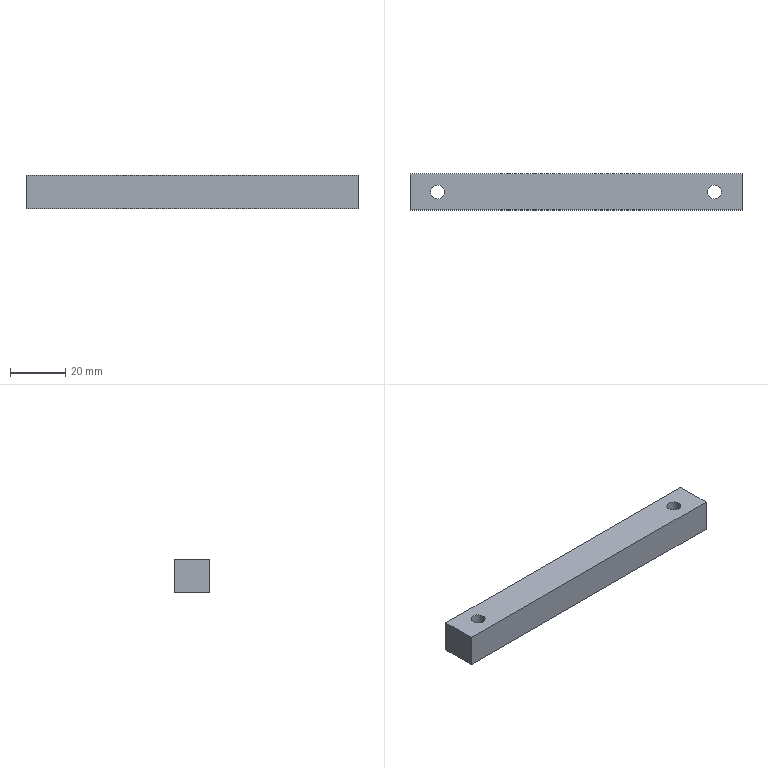Part | STEP file | [14] | 1 solid | 10 faces | box 120 x 13 x 12 mm | volume 18249 mm3 | plane 6 | cylinder 4 | commonest cylinder face diameters 5 x4
STEP:
#1=CARTESIAN_POINT('',(107.5,6.5,12.));
#2=VERTEX_POINT('',#1);
#3=CARTESIAN_POINT('',(112.5,6.5,12.));
#4=VERTEX_POINT('',#3);
#5=CARTESIAN_POINT('',(110.,6.5,12.));
#6=DIRECTION('',(0.,0.,-1.));
#7=DIRECTION('',(1.,0.,0.));
#8=AXIS2_PLACEMENT_3D('',#5,#6,#7);
#9=CIRCLE('',#8,2.5);
#10=EDGE_CURVE('',#2,#4,#9,.T.);
#11=ORIENTED_EDGE('',*,*,#10,.F.);
#12=CARTESIAN_POINT('',(107.5,6.5,0.));
#13=VERTEX_POINT('',#12);
#14=CARTESIAN_POINT('',(107.5,6.5,12.));
#15=DIRECTION('',(0.,0.,-1.));
#16=VECTOR('',#15,1000.);
#17=LINE('',#14,#16);
#18=EDGE_CURVE('',#2,#13,#17,.T.);
#19=ORIENTED_EDGE('',*,*,#18,.T.);
#20=CARTESIAN_POINT('',(112.5,6.5,0.));
#21=VERTEX_POINT('',#20);
#22=CARTESIAN_POINT('',(110.,6.5,0.));
#23=DIRECTION('',(0.,0.,1.));
#24=DIRECTION('',(-1.,0.,0.));
#25=AXIS2_PLACEMENT_3D('',#22,#23,#24);
#26=CIRCLE('',#25,2.5);
#27=EDGE_CURVE('',#21,#13,#26,.T.);
#28=ORIENTED_EDGE('',*,*,#27,.F.);
#29=CARTESIAN_POINT('',(112.5,6.5,12.));
#30=DIRECTION('',(0.,0.,-1.));
#31=VECTOR('',#30,1000.);
#32=LINE('',#29,#31);
#33=EDGE_CURVE('',#4,#21,#32,.T.);
#34=ORIENTED_EDGE('',*,*,#33,.F.);
#35=EDGE_LOOP('',(#11,#19,#28,#34));
#36=FACE_OUTER_BOUND('',#35,.T.);
#37=CARTESIAN_POINT('',(110.,6.5,12.));
#38=DIRECTION('',(0.,0.,-1.));
#39=DIRECTION('',(1.,0.,0.));
#40=AXIS2_PLACEMENT_3D('',#37,#38,#39);
#41=CYLINDRICAL_SURFACE('',#40,2.5);
#42=ADVANCED_FACE('',(#36),#41,.F.);
#43=CARTESIAN_POINT('',(7.5,6.5,12.));
#44=VERTEX_POINT('',#43);
#45=CARTESIAN_POINT('',(12.5,6.5,12.));
#46=VERTEX_POINT('',#45);
#47=CARTESIAN_POINT('',(10.,6.5,12.));
#48=DIRECTION('',(0.,0.,-1.));
#49=DIRECTION('',(1.,0.,0.));
#50=AXIS2_PLACEMENT_3D('',#47,#48,#49);
#51=CIRCLE('',#50,2.5);
#52=EDGE_CURVE('',#44,#46,#51,.T.);
#53=ORIENTED_EDGE('',*,*,#52,.F.);
#54=CARTESIAN_POINT('',(7.5,6.5,0.));
#55=VERTEX_POINT('',#54);
#56=CARTESIAN_POINT('',(7.5,6.5,12.));
#57=DIRECTION('',(0.,0.,-1.));
#58=VECTOR('',#57,1000.);
#59=LINE('',#56,#58);
#60=EDGE_CURVE('',#44,#55,#59,.T.);
#61=ORIENTED_EDGE('',*,*,#60,.T.);
#62=CARTESIAN_POINT('',(12.5,6.5,0.));
#63=VERTEX_POINT('',#62);
#64=CARTESIAN_POINT('',(10.,6.5,0.));
#65=DIRECTION('',(0.,0.,1.));
#66=DIRECTION('',(-1.,0.,0.));
#67=AXIS2_PLACEMENT_3D('',#64,#65,#66);
#68=CIRCLE('',#67,2.5);
#69=EDGE_CURVE('',#63,#55,#68,.T.);
#70=ORIENTED_EDGE('',*,*,#69,.F.);
#71=CARTESIAN_POINT('',(12.5,6.5,12.));
#72=DIRECTION('',(0.,0.,-1.));
#73=VECTOR('',#72,1000.);
#74=LINE('',#71,#73);
#75=EDGE_CURVE('',#46,#63,#74,.T.);
#76=ORIENTED_EDGE('',*,*,#75,.F.);
#77=EDGE_LOOP('',(#53,#61,#70,#76));
#78=FACE_OUTER_BOUND('',#77,.T.);
#79=CARTESIAN_POINT('',(10.,6.5,12.));
#80=DIRECTION('',(0.,0.,-1.));
#81=DIRECTION('',(1.,0.,0.));
#82=AXIS2_PLACEMENT_3D('',#79,#80,#81);
#83=CYLINDRICAL_SURFACE('',#82,2.5);
#84=ADVANCED_FACE('',(#78),#83,.F.);
#85=CARTESIAN_POINT('',(0.,13.,0.));
#86=VERTEX_POINT('',#85);
#87=CARTESIAN_POINT('',(0.,13.,12.));
#88=VERTEX_POINT('',#87);
#89=CARTESIAN_POINT('',(0.,13.,6.));
#90=DIRECTION('',(0.,0.,1.));
#91=VECTOR('',#90,1000.);
#92=LINE('',#89,#91);
#93=EDGE_CURVE('',#86,#88,#92,.T.);
#94=ORIENTED_EDGE('',*,*,#93,.F.);
#95=CARTESIAN_POINT('',(0.,0.,0.));
#96=VERTEX_POINT('',#95);
#97=CARTESIAN_POINT('',(0.,6.5,0.));
#98=DIRECTION('',(0.,1.,0.));
#99=VECTOR('',#98,1000.);
#100=LINE('',#97,#99);
#101=EDGE_CURVE('',#96,#86,#100,.T.);
#102=ORIENTED_EDGE('',*,*,#101,.F.);
#103=CARTESIAN_POINT('',(0.,0.,12.));
#104=VERTEX_POINT('',#103);
#105=CARTESIAN_POINT('',(0.,0.,6.));
#106=DIRECTION('',(0.,0.,-1.));
#107=VECTOR('',#106,1000.);
#108=LINE('',#105,#107);
#109=EDGE_CURVE('',#104,#96,#108,.T.);
#110=ORIENTED_EDGE('',*,*,#109,.F.);
#111=CARTESIAN_POINT('',(0.,6.5,12.));
#112=DIRECTION('',(0.,-1.,0.));
#113=VECTOR('',#112,1000.);
#114=LINE('',#111,#113);
#115=EDGE_CURVE('',#88,#104,#114,.T.);
#116=ORIENTED_EDGE('',*,*,#115,.F.);
#117=EDGE_LOOP('',(#94,#102,#110,#116));
#118=FACE_OUTER_BOUND('',#117,.T.);
#119=CARTESIAN_POINT('',(0.,6.5,6.));
#120=DIRECTION('',(-1.,0.,0.));
#121=DIRECTION('',(0.,0.,-1.));
#122=AXIS2_PLACEMENT_3D('',#119,#120,#121);
#123=PLANE('',#122);
#124=ADVANCED_FACE('',(#118),#123,.T.);
#125=CARTESIAN_POINT('',(120.,13.,0.));
#126=VERTEX_POINT('',#125);
#127=CARTESIAN_POINT('',(120.,13.,0.));
#128=DIRECTION('',(-1.,0.,0.));
#129=VECTOR('',#128,1000.);
#130=LINE('',#127,#129);
#131=EDGE_CURVE('',#126,#86,#130,.T.);
#132=ORIENTED_EDGE('',*,*,#131,.T.);
#133=ORIENTED_EDGE('',*,*,#93,.T.);
#134=CARTESIAN_POINT('',(120.,13.,12.));
#135=VERTEX_POINT('',#134);
#136=CARTESIAN_POINT('',(120.,13.,12.));
#137=DIRECTION('',(-1.,0.,0.));
#138=VECTOR('',#137,1000.);
#139=LINE('',#136,#138);
#140=EDGE_CURVE('',#135,#88,#139,.T.);
#141=ORIENTED_EDGE('',*,*,#140,.F.);
#142=CARTESIAN_POINT('',(120.,13.,6.));
#143=DIRECTION('',(0.,0.,-1.));
#144=VECTOR('',#143,1000.);
#145=LINE('',#142,#144);
#146=EDGE_CURVE('',#135,#126,#145,.T.);
#147=ORIENTED_EDGE('',*,*,#146,.T.);
#148=EDGE_LOOP('',(#132,#133,#141,#147));
#149=FACE_OUTER_BOUND('',#148,.T.);
#150=CARTESIAN_POINT('',(120.,13.,6.));
#151=DIRECTION('',(0.,1.,0.));
#152=DIRECTION('',(1.,0.,0.));
#153=AXIS2_PLACEMENT_3D('',#150,#151,#152);
#154=PLANE('',#153);
#155=ADVANCED_FACE('',(#149),#154,.T.);
#156=CARTESIAN_POINT('',(110.,6.5,12.));
#157=DIRECTION('',(0.,0.,-1.));
#158=DIRECTION('',(1.,0.,0.));
#159=AXIS2_PLACEMENT_3D('',#156,#157,#158);
#160=CIRCLE('',#159,2.5);
#161=EDGE_CURVE('',#4,#2,#160,.T.);
#162=ORIENTED_EDGE('',*,*,#161,.T.);
#163=ORIENTED_EDGE('',*,*,#10,.T.);
#164=EDGE_LOOP('',(#162,#163));
#165=FACE_BOUND('',#164,.T.);
#166=CARTESIAN_POINT('',(10.,6.5,12.));
#167=DIRECTION('',(0.,0.,-1.));
#168=DIRECTION('',(1.,0.,0.));
#169=AXIS2_PLACEMENT_3D('',#166,#167,#168);
#170=CIRCLE('',#169,2.5);
#171=EDGE_CURVE('',#46,#44,#170,.T.);
#172=ORIENTED_EDGE('',*,*,#171,.T.);
#173=ORIENTED_EDGE('',*,*,#52,.T.);
#174=EDGE_LOOP('',(#172,#173));
#175=FACE_BOUND('',#174,.T.);
#176=ORIENTED_EDGE('',*,*,#140,.T.);
#177=ORIENTED_EDGE('',*,*,#115,.T.);
#178=CARTESIAN_POINT('',(120.,0.,12.));
#179=VERTEX_POINT('',#178);
#180=CARTESIAN_POINT('',(120.,0.,12.));
#181=DIRECTION('',(-1.,0.,0.));
#182=VECTOR('',#181,1000.);
#183=LINE('',#180,#182);
#184=EDGE_CURVE('',#179,#104,#183,.T.);
#185=ORIENTED_EDGE('',*,*,#184,.F.);
#186=CARTESIAN_POINT('',(120.,6.5,12.));
#187=DIRECTION('',(0.,1.,0.));
#188=VECTOR('',#187,1000.);
#189=LINE('',#186,#188);
#190=EDGE_CURVE('',#179,#135,#189,.T.);
#191=ORIENTED_EDGE('',*,*,#190,.T.);
#192=EDGE_LOOP('',(#176,#177,#185,#191));
#193=FACE_OUTER_BOUND('',#192,.T.);
#194=CARTESIAN_POINT('',(120.,6.5,12.));
#195=DIRECTION('',(0.,0.,1.));
#196=DIRECTION('',(-1.,0.,0.));
#197=AXIS2_PLACEMENT_3D('',#194,#195,#196);
#198=PLANE('',#197);
#199=ADVANCED_FACE('',(#165,#175,#193),#198,.T.);
#200=ORIENTED_EDGE('',*,*,#184,.T.);
#201=ORIENTED_EDGE('',*,*,#109,.T.);
#202=CARTESIAN_POINT('',(120.,0.,0.));
#203=VERTEX_POINT('',#202);
#204=CARTESIAN_POINT('',(120.,0.,0.));
#205=DIRECTION('',(-1.,0.,0.));
#206=VECTOR('',#205,1000.);
#207=LINE('',#204,#206);
#208=EDGE_CURVE('',#203,#96,#207,.T.);
#209=ORIENTED_EDGE('',*,*,#208,.F.);
#210=CARTESIAN_POINT('',(120.,0.,6.));
#211=DIRECTION('',(0.,0.,1.));
#212=VECTOR('',#211,1000.);
#213=LINE('',#210,#212);
#214=EDGE_CURVE('',#203,#179,#213,.T.);
#215=ORIENTED_EDGE('',*,*,#214,.T.);
#216=EDGE_LOOP('',(#200,#201,#209,#215));
#217=FACE_OUTER_BOUND('',#216,.T.);
#218=CARTESIAN_POINT('',(120.,0.,6.));
#219=DIRECTION('',(0.,-1.,0.));
#220=DIRECTION('',(-1.,0.,0.));
#221=AXIS2_PLACEMENT_3D('',#218,#219,#220);
#222=PLANE('',#221);
#223=ADVANCED_FACE('',(#217),#222,.T.);
#224=CARTESIAN_POINT('',(120.,6.5,0.));
#225=DIRECTION('',(0.,-1.,0.));
#226=VECTOR('',#225,1000.);
#227=LINE('',#224,#226);
#228=EDGE_CURVE('',#126,#203,#227,.T.);
#229=ORIENTED_EDGE('',*,*,#228,.F.);
#230=ORIENTED_EDGE('',*,*,#146,.F.);
#231=ORIENTED_EDGE('',*,*,#190,.F.);
#232=ORIENTED_EDGE('',*,*,#214,.F.);
#233=EDGE_LOOP('',(#229,#230,#231,#232));
#234=FACE_OUTER_BOUND('',#233,.T.);
#235=CARTESIAN_POINT('',(120.,6.5,6.));
#236=DIRECTION('',(1.,0.,0.));
#237=DIRECTION('',(0.,0.,1.));
#238=AXIS2_PLACEMENT_3D('',#235,#236,#237);
#239=PLANE('',#238);
#240=ADVANCED_FACE('',(#234),#239,.T.);
#241=ORIENTED_EDGE('',*,*,#27,.T.);
#242=CARTESIAN_POINT('',(110.,6.5,0.));
#243=DIRECTION('',(0.,0.,1.));
#244=DIRECTION('',(-1.,0.,0.));
#245=AXIS2_PLACEMENT_3D('',#242,#243,#244);
#246=CIRCLE('',#245,2.5);
#247=EDGE_CURVE('',#13,#21,#246,.T.);
#248=ORIENTED_EDGE('',*,*,#247,.T.);
#249=EDGE_LOOP('',(#241,#248));
#250=FACE_BOUND('',#249,.T.);
#251=ORIENTED_EDGE('',*,*,#69,.T.);
#252=CARTESIAN_POINT('',(10.,6.5,0.));
#253=DIRECTION('',(0.,0.,1.));
#254=DIRECTION('',(-1.,0.,0.));
#255=AXIS2_PLACEMENT_3D('',#252,#253,#254);
#256=CIRCLE('',#255,2.5);
#257=EDGE_CURVE('',#55,#63,#256,.T.);
#258=ORIENTED_EDGE('',*,*,#257,.T.);
#259=EDGE_LOOP('',(#251,#258));
#260=FACE_BOUND('',#259,.T.);
#261=ORIENTED_EDGE('',*,*,#228,.T.);
#262=ORIENTED_EDGE('',*,*,#208,.T.);
#263=ORIENTED_EDGE('',*,*,#101,.T.);
#264=ORIENTED_EDGE('',*,*,#131,.F.);
#265=EDGE_LOOP('',(#261,#262,#263,#264));
#266=FACE_OUTER_BOUND('',#265,.T.);
#267=CARTESIAN_POINT('',(120.,6.5,0.));
#268=DIRECTION('',(0.,0.,-1.));
#269=DIRECTION('',(1.,0.,0.));
#270=AXIS2_PLACEMENT_3D('',#267,#268,#269);
#271=PLANE('',#270);
#272=ADVANCED_FACE('',(#250,#260,#266),#271,.T.);
#273=ORIENTED_EDGE('',*,*,#60,.F.);
#274=ORIENTED_EDGE('',*,*,#171,.F.);
#275=ORIENTED_EDGE('',*,*,#75,.T.);
#276=ORIENTED_EDGE('',*,*,#257,.F.);
#277=EDGE_LOOP('',(#273,#274,#275,#276));
#278=FACE_OUTER_BOUND('',#277,.T.);
#279=CARTESIAN_POINT('',(10.,6.5,12.));
#280=DIRECTION('',(0.,0.,-1.));
#281=DIRECTION('',(1.,0.,0.));
#282=AXIS2_PLACEMENT_3D('',#279,#280,#281);
#283=CYLINDRICAL_SURFACE('',#282,2.5);
#284=ADVANCED_FACE('',(#278),#283,.F.);
#285=ORIENTED_EDGE('',*,*,#18,.F.);
#286=ORIENTED_EDGE('',*,*,#161,.F.);
#287=ORIENTED_EDGE('',*,*,#33,.T.);
#288=ORIENTED_EDGE('',*,*,#247,.F.);
#289=EDGE_LOOP('',(#285,#286,#287,#288));
#290=FACE_OUTER_BOUND('',#289,.T.);
#291=CARTESIAN_POINT('',(110.,6.5,12.));
#292=DIRECTION('',(0.,0.,-1.));
#293=DIRECTION('',(1.,0.,0.));
#294=AXIS2_PLACEMENT_3D('',#291,#292,#293);
#295=CYLINDRICAL_SURFACE('',#294,2.5);
#296=ADVANCED_FACE('',(#290),#295,.F.);
#297=CLOSED_SHELL('',(#42,#84,#124,#155,#199,#223,#240,#272,#284,#296));
#298=MANIFOLD_SOLID_BREP('',#297);
#299=CARTESIAN_POINT('',(0.,0.,0.));
#300=DIRECTION('',(0.,0.,1.));
#301=DIRECTION('',(1.,0.,0.));
#302=AXIS2_PLACEMENT_3D('',#299,#300,#301);
#303=(LENGTH_UNIT()NAMED_UNIT(*)SI_UNIT(.MILLI.,.METRE.));
#304=UNCERTAINTY_MEASURE_WITH_UNIT(LENGTH_MEASURE(0.00001),#303,'','');
#305=(NAMED_UNIT(*)PLANE_ANGLE_UNIT()SI_UNIT($,.RADIAN.));
#306=(NAMED_UNIT(*)SI_UNIT($,.STERADIAN.)SOLID_ANGLE_UNIT());
#307=(GEOMETRIC_REPRESENTATION_CONTEXT(3)GLOBAL_UNCERTAINTY_ASSIGNED_CONTEXT((#304))GLOBAL_UNIT_ASSIGNED_CONTEXT((#303,#305,#306))REPRESENTATION_CONTEXT('',''));
#308=ADVANCED_BREP_SHAPE_REPRESENTATION('',(#298,#302),#307);